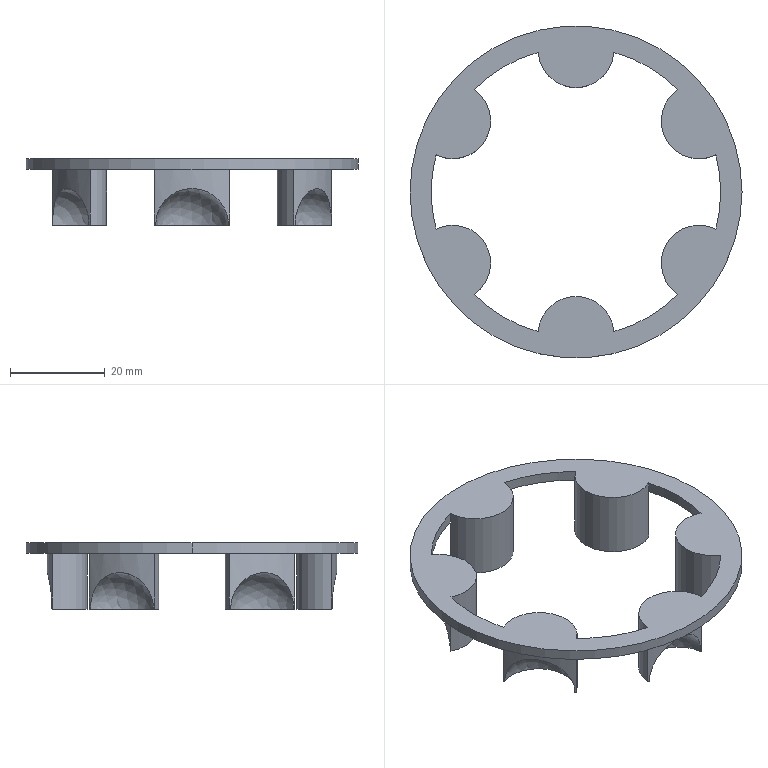Part | NX | features BREP 1 | 1 solid | 37 faces | box 70 x 70 x 14 mm | volume 7900 mm3 | cylinder 23 | plane 8 | sphere 6 | commonest cylinder face diameters 61 x13 16 x8 70 x2
STEP:
#1=CARTESIAN_POINT('',(26.414,15.25,-4.05));
#2=VERTEX_POINT('',#1);
#3=CARTESIAN_POINT('',(21.717,21.415,-11.8));
#4=VERTEX_POINT('',#3);
#5=CARTESIAN_POINT('',(21.717,21.415,-11.8));
#6=CARTESIAN_POINT('',(21.717,21.415,-9.751));
#7=CARTESIAN_POINT('',(22.961,20.244,-5.743));
#8=CARTESIAN_POINT('',(25.389,17.025,-4.05));
#9=CARTESIAN_POINT('',(26.414,15.25,-4.05));
#10=B_SPLINE_CURVE_WITH_KNOTS('',3,(#5,#6,#7,#8,#9),.UNSPECIFIED.,.F.,.F.,(4,1,4),(0.,0.00606,0.01212),.UNSPECIFIED.);
#11=EDGE_CURVE('',#2,#4,#10,.F.);
#12=ORIENTED_EDGE('',*,*,#11,.T.);
#13=CARTESIAN_POINT('',(21.504,21.63,-11.8));
#14=VERTEX_POINT('',#13);
#15=CARTESIAN_POINT('',(0.,0.,-11.8));
#16=DIRECTION('',(0.,0.,-1.));
#17=DIRECTION('',(0.705,0.7092,0.));
#18=AXIS2_PLACEMENT_3D('',#15,#16,#17);
#19=CIRCLE('',#18,30.5);
#20=EDGE_CURVE('',#14,#4,#19,.T.);
#21=ORIENTED_EDGE('',*,*,#20,.F.);
#22=CARTESIAN_POINT('',(21.504,21.63,0.));
#23=VERTEX_POINT('',#22);
#24=CARTESIAN_POINT('',(21.504,21.63,0.));
#25=DIRECTION('',(0.,0.,-1.));
#26=VECTOR('',#25,1000.);
#27=LINE('',#24,#26);
#28=EDGE_CURVE('',#23,#14,#27,.T.);
#29=ORIENTED_EDGE('',*,*,#28,.F.);
#30=CARTESIAN_POINT('',(29.484,7.808,0.));
#31=VERTEX_POINT('',#30);
#32=CARTESIAN_POINT('',(0.,0.,0.));
#33=DIRECTION('',(0.,0.,1.));
#34=DIRECTION('',(0.9667,0.256,0.));
#35=AXIS2_PLACEMENT_3D('',#32,#33,#34);
#36=CIRCLE('',#35,30.5);
#37=EDGE_CURVE('',#31,#23,#36,.T.);
#38=ORIENTED_EDGE('',*,*,#37,.F.);
#39=CARTESIAN_POINT('',(29.484,7.808,-11.8));
#40=VERTEX_POINT('',#39);
#41=CARTESIAN_POINT('',(29.484,7.808,0.));
#42=DIRECTION('',(0.,0.,-1.));
#43=VECTOR('',#42,1000.);
#44=LINE('',#41,#43);
#45=EDGE_CURVE('',#31,#40,#44,.T.);
#46=ORIENTED_EDGE('',*,*,#45,.T.);
#47=CARTESIAN_POINT('',(29.405,8.1,-11.8));
#48=VERTEX_POINT('',#47);
#49=CARTESIAN_POINT('',(0.,0.,-11.8));
#50=DIRECTION('',(0.,0.,-1.));
#51=DIRECTION('',(0.9641,0.2656,0.));
#52=AXIS2_PLACEMENT_3D('',#49,#50,#51);
#53=CIRCLE('',#52,30.5);
#54=EDGE_CURVE('',#48,#40,#53,.T.);
#55=ORIENTED_EDGE('',*,*,#54,.F.);
#56=CARTESIAN_POINT('',(29.405,8.1,-11.8));
#57=CARTESIAN_POINT('',(29.405,8.1,-9.751));
#58=CARTESIAN_POINT('',(29.012,9.763,-5.743));
#59=CARTESIAN_POINT('',(27.439,13.475,-4.05));
#60=CARTESIAN_POINT('',(26.414,15.25,-4.05));
#61=B_SPLINE_CURVE_WITH_KNOTS('',3,(#56,#57,#58,#59,#60),.UNSPECIFIED.,.F.,.F.,(4,1,4),(0.,0.00606,0.01212),.UNSPECIFIED.);
#62=EDGE_CURVE('',#2,#48,#61,.F.);
#63=ORIENTED_EDGE('',*,*,#62,.F.);
#64=EDGE_LOOP('',(#12,#21,#29,#38,#46,#55,#63));
#65=FACE_BOUND('',#64,.T.);
#66=CARTESIAN_POINT('',(0.,0.,-11.8));
#67=DIRECTION('',(0.,0.,1.));
#68=DIRECTION('',(-1.,0.,0.));
#69=AXIS2_PLACEMENT_3D('',#66,#67,#68);
#70=CYLINDRICAL_SURFACE('',#69,30.5);
#71=ADVANCED_FACE('',(#65),#70,.T.);
#72=ORIENTED_EDGE('',*,*,#62,.T.);
#73=CARTESIAN_POINT('',(18.664,15.25,-11.8));
#74=VERTEX_POINT('',#73);
#75=CARTESIAN_POINT('',(26.414,15.25,-11.8));
#76=DIRECTION('',(0.,0.,1.));
#77=DIRECTION('',(-1.,0.,0.));
#78=AXIS2_PLACEMENT_3D('',#75,#76,#77);
#79=CIRCLE('',#78,7.75);
#80=EDGE_CURVE('',#74,#48,#79,.T.);
#81=ORIENTED_EDGE('',*,*,#80,.F.);
#82=CARTESIAN_POINT('',(26.414,15.25,-11.8));
#83=DIRECTION('',(0.,0.,1.));
#84=DIRECTION('',(-0.606,0.7955,0.));
#85=AXIS2_PLACEMENT_3D('',#82,#83,#84);
#86=CIRCLE('',#85,7.75);
#87=EDGE_CURVE('',#4,#74,#86,.T.);
#88=ORIENTED_EDGE('',*,*,#87,.F.);
#89=ORIENTED_EDGE('',*,*,#11,.F.);
#90=EDGE_LOOP('',(#72,#81,#88,#89));
#91=FACE_BOUND('',#90,.T.);
#92=CARTESIAN_POINT('',(26.414,15.25,-11.8));
#93=DIRECTION('',(0.3859,-0.9225,0.));
#94=DIRECTION('',(0.,0.,1.));
#95=AXIS2_PLACEMENT_3D('',#92,#93,#94);
#96=SPHERICAL_SURFACE('',#95,7.75);
#97=ADVANCED_FACE('',(#91),#96,.F.);
#98=ORIENTED_EDGE('',*,*,#87,.T.);
#99=ORIENTED_EDGE('',*,*,#80,.T.);
#100=ORIENTED_EDGE('',*,*,#54,.T.);
#101=CARTESIAN_POINT('',(17.981,15.,-11.8));
#102=VERTEX_POINT('',#101);
#103=CARTESIAN_POINT('',(25.981,15.,-11.8));
#104=DIRECTION('',(0.,0.,-1.));
#105=DIRECTION('',(0.4379,-0.899,0.));
#106=AXIS2_PLACEMENT_3D('',#103,#104,#105);
#107=CIRCLE('',#106,8.);
#108=EDGE_CURVE('',#40,#102,#107,.T.);
#109=ORIENTED_EDGE('',*,*,#108,.T.);
#110=CARTESIAN_POINT('',(25.981,15.,-11.8));
#111=DIRECTION('',(0.,0.,-1.));
#112=DIRECTION('',(-1.,0.,0.));
#113=AXIS2_PLACEMENT_3D('',#110,#111,#112);
#114=CIRCLE('',#113,8.);
#115=EDGE_CURVE('',#102,#14,#114,.T.);
#116=ORIENTED_EDGE('',*,*,#115,.T.);
#117=ORIENTED_EDGE('',*,*,#20,.T.);
#118=EDGE_LOOP('',(#98,#99,#100,#109,#116,#117));
#119=FACE_BOUND('',#118,.T.);
#120=CARTESIAN_POINT('',(12.99,7.5,-11.8));
#121=DIRECTION('',(0.,0.,1.));
#122=DIRECTION('',(-1.,0.,0.));
#123=AXIS2_PLACEMENT_3D('',#120,#121,#122);
#124=PLANE('',#123);
#125=ADVANCED_FACE('',(#119),#124,.F.);
#126=CARTESIAN_POINT('',(21.504,21.63,2.2));
#127=VERTEX_POINT('',#126);
#128=CARTESIAN_POINT('',(17.981,15.,2.2));
#129=VERTEX_POINT('',#128);
#130=CARTESIAN_POINT('',(25.981,15.,2.2));
#131=DIRECTION('',(0.,0.,1.));
#132=DIRECTION('',(-0.5597,0.8287,0.));
#133=AXIS2_PLACEMENT_3D('',#130,#131,#132);
#134=CIRCLE('',#133,8.);
#135=EDGE_CURVE('',#127,#129,#134,.T.);
#136=ORIENTED_EDGE('',*,*,#135,.F.);
#137=CARTESIAN_POINT('',(21.504,21.63,0.));
#138=DIRECTION('',(0.,0.,1.));
#139=VECTOR('',#138,1000.);
#140=LINE('',#137,#139);
#141=EDGE_CURVE('',#23,#127,#140,.T.);
#142=ORIENTED_EDGE('',*,*,#141,.F.);
#143=ORIENTED_EDGE('',*,*,#28,.T.);
#144=ORIENTED_EDGE('',*,*,#115,.F.);
#145=CARTESIAN_POINT('',(17.981,15.,-11.8));
#146=DIRECTION('',(0.,0.,1.));
#147=VECTOR('',#146,1000.);
#148=LINE('',#145,#147);
#149=EDGE_CURVE('',#102,#129,#148,.T.);
#150=ORIENTED_EDGE('',*,*,#149,.T.);
#151=EDGE_LOOP('',(#136,#142,#143,#144,#150));
#152=FACE_BOUND('',#151,.T.);
#153=CARTESIAN_POINT('',(25.981,15.,2.2));
#154=DIRECTION('',(0.,0.,-1.));
#155=DIRECTION('',(1.,0.,0.));
#156=AXIS2_PLACEMENT_3D('',#153,#154,#155);
#157=CYLINDRICAL_SURFACE('',#156,8.);
#158=ADVANCED_FACE('',(#152),#157,.T.);
#159=ORIENTED_EDGE('',*,*,#149,.F.);
#160=ORIENTED_EDGE('',*,*,#108,.F.);
#161=ORIENTED_EDGE('',*,*,#45,.F.);
#162=CARTESIAN_POINT('',(29.484,7.808,2.2));
#163=VERTEX_POINT('',#162);
#164=CARTESIAN_POINT('',(29.484,7.808,0.));
#165=DIRECTION('',(0.,0.,1.));
#166=VECTOR('',#165,1000.);
#167=LINE('',#164,#166);
#168=EDGE_CURVE('',#31,#163,#167,.T.);
#169=ORIENTED_EDGE('',*,*,#168,.T.);
#170=CARTESIAN_POINT('',(25.981,15.,2.2));
#171=DIRECTION('',(0.,0.,1.));
#172=DIRECTION('',(-1.,0.,0.));
#173=AXIS2_PLACEMENT_3D('',#170,#171,#172);
#174=CIRCLE('',#173,8.);
#175=EDGE_CURVE('',#129,#163,#174,.T.);
#176=ORIENTED_EDGE('',*,*,#175,.F.);
#177=EDGE_LOOP('',(#159,#160,#161,#169,#176));
#178=FACE_BOUND('',#177,.T.);
#179=CARTESIAN_POINT('',(25.981,15.,2.2));
#180=DIRECTION('',(0.,0.,-1.));
#181=DIRECTION('',(1.,0.,0.));
#182=AXIS2_PLACEMENT_3D('',#179,#180,#181);
#183=CYLINDRICAL_SURFACE('',#182,8.);
#184=ADVANCED_FACE('',(#178),#183,.T.);
#185=CARTESIAN_POINT('',(35.,0.,2.2));
#186=VERTEX_POINT('',#185);
#187=CARTESIAN_POINT('',(-35.,0.,2.2));
#188=VERTEX_POINT('',#187);
#189=CARTESIAN_POINT('',(0.,0.,2.2));
#190=DIRECTION('',(0.,0.,1.));
#191=DIRECTION('',(1.,0.,0.));
#192=AXIS2_PLACEMENT_3D('',#189,#190,#191);
#193=CIRCLE('',#192,35.);
#194=EDGE_CURVE('',#186,#188,#193,.T.);
#195=ORIENTED_EDGE('',*,*,#194,.T.);
#196=CARTESIAN_POINT('',(0.,0.,2.2));
#197=DIRECTION('',(0.,0.,1.));
#198=DIRECTION('',(-1.,0.,0.));
#199=AXIS2_PLACEMENT_3D('',#196,#197,#198);
#200=CIRCLE('',#199,35.);
#201=EDGE_CURVE('',#188,#186,#200,.T.);
#202=ORIENTED_EDGE('',*,*,#201,.T.);
#203=EDGE_LOOP('',(#195,#202));
#204=FACE_BOUND('',#203,.T.);
#205=CARTESIAN_POINT('',(-29.484,7.808,2.2));
#206=VERTEX_POINT('',#205);
#207=CARTESIAN_POINT('',(-21.504,21.63,2.2));
#208=VERTEX_POINT('',#207);
#209=CARTESIAN_POINT('',(-25.981,15.,2.2));
#210=DIRECTION('',(0.,0.,1.));
#211=DIRECTION('',(-0.4379,-0.899,0.));
#212=AXIS2_PLACEMENT_3D('',#209,#210,#211);
#213=CIRCLE('',#212,8.);
#214=EDGE_CURVE('',#206,#208,#213,.T.);
#215=ORIENTED_EDGE('',*,*,#214,.T.);
#216=CARTESIAN_POINT('',(-7.98,29.438,2.2));
#217=VERTEX_POINT('',#216);
#218=CARTESIAN_POINT('',(0.,0.,2.2));
#219=DIRECTION('',(0.,0.,-1.));
#220=DIRECTION('',(-0.705,0.7092,0.));
#221=AXIS2_PLACEMENT_3D('',#218,#219,#220);
#222=CIRCLE('',#221,30.5);
#223=EDGE_CURVE('',#208,#217,#222,.T.);
#224=ORIENTED_EDGE('',*,*,#223,.T.);
#225=CARTESIAN_POINT('',(7.98,29.438,2.2));
#226=VERTEX_POINT('',#225);
#227=CARTESIAN_POINT('',(0.,30.,2.2));
#228=DIRECTION('',(0.,0.,1.));
#229=DIRECTION('',(-0.9975,-0.07031,0.));
#230=AXIS2_PLACEMENT_3D('',#227,#228,#229);
#231=CIRCLE('',#230,8.);
#232=EDGE_CURVE('',#217,#226,#231,.T.);
#233=ORIENTED_EDGE('',*,*,#232,.T.);
#234=CARTESIAN_POINT('',(0.,0.,2.2));
#235=DIRECTION('',(0.,0.,-1.));
#236=DIRECTION('',(0.2616,0.9652,0.));
#237=AXIS2_PLACEMENT_3D('',#234,#235,#236);
#238=CIRCLE('',#237,30.5);
#239=EDGE_CURVE('',#226,#127,#238,.T.);
#240=ORIENTED_EDGE('',*,*,#239,.T.);
#241=ORIENTED_EDGE('',*,*,#135,.T.);
#242=ORIENTED_EDGE('',*,*,#175,.T.);
#243=CARTESIAN_POINT('',(29.484,-7.808,2.2));
#244=VERTEX_POINT('',#243);
#245=CARTESIAN_POINT('',(0.,0.,2.2));
#246=DIRECTION('',(0.,0.,-1.));
#247=DIRECTION('',(0.9667,0.256,0.));
#248=AXIS2_PLACEMENT_3D('',#245,#246,#247);
#249=CIRCLE('',#248,30.5);
#250=EDGE_CURVE('',#163,#244,#249,.T.);
#251=ORIENTED_EDGE('',*,*,#250,.T.);
#252=CARTESIAN_POINT('',(17.981,-15.,2.2));
#253=VERTEX_POINT('',#252);
#254=CARTESIAN_POINT('',(25.981,-15.,2.2));
#255=DIRECTION('',(0.,0.,1.));
#256=DIRECTION('',(0.4379,0.899,0.));
#257=AXIS2_PLACEMENT_3D('',#254,#255,#256);
#258=CIRCLE('',#257,8.);
#259=EDGE_CURVE('',#244,#253,#258,.T.);
#260=ORIENTED_EDGE('',*,*,#259,.T.);
#261=CARTESIAN_POINT('',(21.504,-21.63,2.2));
#262=VERTEX_POINT('',#261);
#263=CARTESIAN_POINT('',(25.981,-15.,2.2));
#264=DIRECTION('',(0.,0.,1.));
#265=DIRECTION('',(-1.,0.,0.));
#266=AXIS2_PLACEMENT_3D('',#263,#264,#265);
#267=CIRCLE('',#266,8.);
#268=EDGE_CURVE('',#253,#262,#267,.T.);
#269=ORIENTED_EDGE('',*,*,#268,.T.);
#270=CARTESIAN_POINT('',(7.98,-29.438,2.2));
#271=VERTEX_POINT('',#270);
#272=CARTESIAN_POINT('',(0.,0.,2.2));
#273=DIRECTION('',(0.,0.,-1.));
#274=DIRECTION('',(0.705,-0.7092,0.));
#275=AXIS2_PLACEMENT_3D('',#272,#273,#274);
#276=CIRCLE('',#275,30.5);
#277=EDGE_CURVE('',#262,#271,#276,.T.);
#278=ORIENTED_EDGE('',*,*,#277,.T.);
#279=CARTESIAN_POINT('',(-7.98,-29.438,2.2));
#280=VERTEX_POINT('',#279);
#281=CARTESIAN_POINT('',(0.,-30.,2.2));
#282=DIRECTION('',(0.,0.,1.));
#283=DIRECTION('',(0.9975,0.07031,0.));
#284=AXIS2_PLACEMENT_3D('',#281,#282,#283);
#285=CIRCLE('',#284,8.);
#286=EDGE_CURVE('',#271,#280,#285,.T.);
#287=ORIENTED_EDGE('',*,*,#286,.T.);
#288=CARTESIAN_POINT('',(-21.504,-21.63,2.2));
#289=VERTEX_POINT('',#288);
#290=CARTESIAN_POINT('',(0.,0.,2.2));
#291=DIRECTION('',(0.,0.,-1.));
#292=DIRECTION('',(-0.2616,-0.9652,0.));
#293=AXIS2_PLACEMENT_3D('',#290,#291,#292);
#294=CIRCLE('',#293,30.5);
#295=EDGE_CURVE('',#280,#289,#294,.T.);
#296=ORIENTED_EDGE('',*,*,#295,.T.);
#297=CARTESIAN_POINT('',(-29.484,-7.808,2.2));
#298=VERTEX_POINT('',#297);
#299=CARTESIAN_POINT('',(-25.981,-15.,2.2));
#300=DIRECTION('',(0.,0.,1.));
#301=DIRECTION('',(0.5597,-0.8287,0.));
#302=AXIS2_PLACEMENT_3D('',#299,#300,#301);
#303=CIRCLE('',#302,8.);
#304=EDGE_CURVE('',#289,#298,#303,.T.);
#305=ORIENTED_EDGE('',*,*,#304,.T.);
#306=CARTESIAN_POINT('',(-30.5,0.,2.2));
#307=VERTEX_POINT('',#306);
#308=CARTESIAN_POINT('',(0.,0.,2.2));
#309=DIRECTION('',(0.,0.,-1.));
#310=DIRECTION('',(-0.9667,-0.256,0.));
#311=AXIS2_PLACEMENT_3D('',#308,#309,#310);
#312=CIRCLE('',#311,30.5);
#313=EDGE_CURVE('',#298,#307,#312,.T.);
#314=ORIENTED_EDGE('',*,*,#313,.T.);
#315=CARTESIAN_POINT('',(0.,0.,2.2));
#316=DIRECTION('',(0.,0.,-1.));
#317=DIRECTION('',(-1.,0.,0.));
#318=AXIS2_PLACEMENT_3D('',#315,#316,#317);
#319=CIRCLE('',#318,30.5);
#320=EDGE_CURVE('',#307,#206,#319,.T.);
#321=ORIENTED_EDGE('',*,*,#320,.T.);
#322=EDGE_LOOP('',(#215,#224,#233,#240,#241,#242,#251,#260,#269,#278,#287,#296,#305,#314,#321));
#323=FACE_BOUND('',#322,.T.);
#324=CARTESIAN_POINT('',(0.,0.,2.2));
#325=DIRECTION('',(0.,0.,1.));
#326=DIRECTION('',(-1.,0.,0.));
#327=AXIS2_PLACEMENT_3D('',#324,#325,#326);
#328=PLANE('',#327);
#329=ADVANCED_FACE('',(#204,#323),#328,.T.);
#330=ORIENTED_EDGE('',*,*,#201,.F.);
#331=CARTESIAN_POINT('',(-35.,0.,0.));
#332=VERTEX_POINT('',#331);
#333=CARTESIAN_POINT('',(-35.,0.,0.));
#334=DIRECTION('',(0.,0.,1.));
#335=VECTOR('',#334,1000.);
#336=LINE('',#333,#335);
#337=EDGE_CURVE('',#188,#332,#336,.F.);
#338=ORIENTED_EDGE('',*,*,#337,.T.);
#339=CARTESIAN_POINT('',(35.,0.,0.));
#340=VERTEX_POINT('',#339);
#341=CARTESIAN_POINT('',(0.,0.,0.));
#342=DIRECTION('',(0.,0.,-1.));
#343=DIRECTION('',(1.,0.,0.));
#344=AXIS2_PLACEMENT_3D('',#341,#342,#343);
#345=CIRCLE('',#344,35.);
#346=EDGE_CURVE('',#340,#332,#345,.T.);
#347=ORIENTED_EDGE('',*,*,#346,.F.);
#348=CARTESIAN_POINT('',(35.,0.,0.));
#349=DIRECTION('',(0.,0.,1.));
#350=VECTOR('',#349,1000.);
#351=LINE('',#348,#350);
#352=EDGE_CURVE('',#186,#340,#351,.F.);
#353=ORIENTED_EDGE('',*,*,#352,.F.);
#354=EDGE_LOOP('',(#330,#338,#347,#353));
#355=FACE_BOUND('',#354,.T.);
#356=CARTESIAN_POINT('',(0.,0.,2.2));
#357=DIRECTION('',(0.,0.,-1.));
#358=DIRECTION('',(1.,0.,0.));
#359=AXIS2_PLACEMENT_3D('',#356,#357,#358);
#360=CYLINDRICAL_SURFACE('',#359,35.);
#361=ADVANCED_FACE('',(#355),#360,.T.);
#362=ORIENTED_EDGE('',*,*,#352,.T.);
#363=CARTESIAN_POINT('',(0.,0.,0.));
#364=DIRECTION('',(0.,0.,-1.));
#365=DIRECTION('',(-1.,0.,0.));
#366=AXIS2_PLACEMENT_3D('',#363,#364,#365);
#367=CIRCLE('',#366,35.);
#368=EDGE_CURVE('',#332,#340,#367,.T.);
#369=ORIENTED_EDGE('',*,*,#368,.F.);
#370=ORIENTED_EDGE('',*,*,#337,.F.);
#371=ORIENTED_EDGE('',*,*,#194,.F.);
#372=EDGE_LOOP('',(#362,#369,#370,#371));
#373=FACE_BOUND('',#372,.T.);
#374=CARTESIAN_POINT('',(0.,0.,2.2));
#375=DIRECTION('',(0.,0.,-1.));
#376=DIRECTION('',(1.,0.,0.));
#377=AXIS2_PLACEMENT_3D('',#374,#375,#376);
#378=CYLINDRICAL_SURFACE('',#377,35.);
#379=ADVANCED_FACE('',(#373),#378,.T.);
#380=ORIENTED_EDGE('',*,*,#368,.T.);
#381=ORIENTED_EDGE('',*,*,#346,.T.);
#382=EDGE_LOOP('',(#380,#381));
#383=FACE_BOUND('',#382,.T.);
#384=CARTESIAN_POINT('',(-21.504,21.63,0.));
#385=VERTEX_POINT('',#384);
#386=CARTESIAN_POINT('',(-29.484,7.808,0.));
#387=VERTEX_POINT('',#386);
#388=CARTESIAN_POINT('',(0.,0.,0.));
#389=DIRECTION('',(0.,0.,1.));
#390=DIRECTION('',(-0.705,0.7092,0.));
#391=AXIS2_PLACEMENT_3D('',#388,#389,#390);
#392=CIRCLE('',#391,30.5);
#393=EDGE_CURVE('',#385,#387,#392,.T.);
#394=ORIENTED_EDGE('',*,*,#393,.T.);
#395=CARTESIAN_POINT('',(-30.5,0.,0.));
#396=VERTEX_POINT('',#395);
#397=CARTESIAN_POINT('',(0.,0.,0.));
#398=DIRECTION('',(0.,0.,1.));
#399=DIRECTION('',(-0.9667,0.256,0.));
#400=AXIS2_PLACEMENT_3D('',#397,#398,#399);
#401=CIRCLE('',#400,30.5);
#402=EDGE_CURVE('',#387,#396,#401,.T.);
#403=ORIENTED_EDGE('',*,*,#402,.T.);
#404=CARTESIAN_POINT('',(-29.484,-7.808,0.));
#405=VERTEX_POINT('',#404);
#406=CARTESIAN_POINT('',(0.,0.,0.));
#407=DIRECTION('',(0.,0.,1.));
#408=DIRECTION('',(-1.,0.,0.));
#409=AXIS2_PLACEMENT_3D('',#406,#407,#408);
#410=CIRCLE('',#409,30.5);
#411=EDGE_CURVE('',#396,#405,#410,.T.);
#412=ORIENTED_EDGE('',*,*,#411,.T.);
#413=CARTESIAN_POINT('',(-21.504,-21.63,0.));
#414=VERTEX_POINT('',#413);
#415=CARTESIAN_POINT('',(0.,0.,0.));
#416=DIRECTION('',(0.,0.,1.));
#417=DIRECTION('',(-0.9667,-0.256,0.));
#418=AXIS2_PLACEMENT_3D('',#415,#416,#417);
#419=CIRCLE('',#418,30.5);
#420=EDGE_CURVE('',#405,#414,#419,.T.);
#421=ORIENTED_EDGE('',*,*,#420,.T.);
#422=CARTESIAN_POINT('',(-7.98,-29.438,0.));
#423=VERTEX_POINT('',#422);
#424=CARTESIAN_POINT('',(0.,0.,0.));
#425=DIRECTION('',(0.,0.,1.));
#426=DIRECTION('',(-0.705,-0.7092,0.));
#427=AXIS2_PLACEMENT_3D('',#424,#425,#426);
#428=CIRCLE('',#427,30.5);
#429=EDGE_CURVE('',#414,#423,#428,.T.);
#430=ORIENTED_EDGE('',*,*,#429,.T.);
#431=CARTESIAN_POINT('',(7.98,-29.438,0.));
#432=VERTEX_POINT('',#431);
#433=CARTESIAN_POINT('',(0.,0.,0.));
#434=DIRECTION('',(0.,0.,1.));
#435=DIRECTION('',(-0.2616,-0.9652,0.));
#436=AXIS2_PLACEMENT_3D('',#433,#434,#435);
#437=CIRCLE('',#436,30.5);
#438=EDGE_CURVE('',#423,#432,#437,.T.);
#439=ORIENTED_EDGE('',*,*,#438,.T.);
#440=CARTESIAN_POINT('',(21.504,-21.63,0.));
#441=VERTEX_POINT('',#440);
#442=CARTESIAN_POINT('',(0.,0.,0.));
#443=DIRECTION('',(0.,0.,1.));
#444=DIRECTION('',(0.2616,-0.9652,0.));
#445=AXIS2_PLACEMENT_3D('',#442,#443,#444);
#446=CIRCLE('',#445,30.5);
#447=EDGE_CURVE('',#432,#441,#446,.T.);
#448=ORIENTED_EDGE('',*,*,#447,.T.);
#449=CARTESIAN_POINT('',(29.484,-7.808,0.));
#450=VERTEX_POINT('',#449);
#451=CARTESIAN_POINT('',(0.,0.,0.));
#452=DIRECTION('',(0.,0.,1.));
#453=DIRECTION('',(0.705,-0.7092,0.));
#454=AXIS2_PLACEMENT_3D('',#451,#452,#453);
#455=CIRCLE('',#454,30.5);
#456=EDGE_CURVE('',#441,#450,#455,.T.);
#457=ORIENTED_EDGE('',*,*,#456,.T.);
#458=CARTESIAN_POINT('',(0.,0.,0.));
#459=DIRECTION('',(0.,0.,1.));
#460=DIRECTION('',(0.9667,-0.256,0.));
#461=AXIS2_PLACEMENT_3D('',#458,#459,#460);
#462=CIRCLE('',#461,30.5);
#463=EDGE_CURVE('',#450,#31,#462,.T.);
#464=ORIENTED_EDGE('',*,*,#463,.T.);
#465=ORIENTED_EDGE('',*,*,#37,.T.);
#466=CARTESIAN_POINT('',(7.98,29.438,0.));
#467=VERTEX_POINT('',#466);
#468=CARTESIAN_POINT('',(0.,0.,0.));
#469=DIRECTION('',(0.,0.,1.));
#470=DIRECTION('',(0.705,0.7092,0.));
#471=AXIS2_PLACEMENT_3D('',#468,#469,#470);
#472=CIRCLE('',#471,30.5);
#473=EDGE_CURVE('',#23,#467,#472,.T.);
#474=ORIENTED_EDGE('',*,*,#473,.T.);
#475=CARTESIAN_POINT('',(-7.98,29.438,0.));
#476=VERTEX_POINT('',#475);
#477=CARTESIAN_POINT('',(0.,0.,0.));
#478=DIRECTION('',(0.,0.,1.));
#479=DIRECTION('',(0.2616,0.9652,0.));
#480=AXIS2_PLACEMENT_3D('',#477,#478,#479);
#481=CIRCLE('',#480,30.5);
#482=EDGE_CURVE('',#467,#476,#481,.T.);
#483=ORIENTED_EDGE('',*,*,#482,.T.);
#484=CARTESIAN_POINT('',(0.,0.,0.));
#485=DIRECTION('',(0.,0.,1.));
#486=DIRECTION('',(-0.2616,0.9652,0.));
#487=AXIS2_PLACEMENT_3D('',#484,#485,#486);
#488=CIRCLE('',#487,30.5);
#489=EDGE_CURVE('',#476,#385,#488,.T.);
#490=ORIENTED_EDGE('',*,*,#489,.T.);
#491=EDGE_LOOP('',(#394,#403,#412,#421,#430,#439,#448,#457,#464,#465,#474,#483,#490));
#492=FACE_BOUND('',#491,.T.);
#493=CARTESIAN_POINT('',(0.,0.,0.));
#494=DIRECTION('',(0.,0.,1.));
#495=DIRECTION('',(-1.,0.,0.));
#496=AXIS2_PLACEMENT_3D('',#493,#494,#495);
#497=PLANE('',#496);
#498=ADVANCED_FACE('',(#383,#492),#497,.F.);
#499=CARTESIAN_POINT('',(-7.98,29.438,0.));
#500=DIRECTION('',(0.,0.,1.));
#501=VECTOR('',#500,1000.);
#502=LINE('',#499,#501);
#503=EDGE_CURVE('',#476,#217,#502,.T.);
#504=ORIENTED_EDGE('',*,*,#503,.T.);
#505=ORIENTED_EDGE('',*,*,#223,.F.);
#506=CARTESIAN_POINT('',(-21.504,21.63,0.));
#507=DIRECTION('',(0.,0.,1.));
#508=VECTOR('',#507,1000.);
#509=LINE('',#506,#508);
#510=EDGE_CURVE('',#385,#208,#509,.T.);
#511=ORIENTED_EDGE('',*,*,#510,.F.);
#512=ORIENTED_EDGE('',*,*,#489,.F.);
#513=EDGE_LOOP('',(#504,#505,#511,#512));
#514=FACE_BOUND('',#513,.T.);
#515=CARTESIAN_POINT('',(0.,0.,2.2));
#516=DIRECTION('',(0.,0.,-1.));
#517=DIRECTION('',(1.,0.,0.));
#518=AXIS2_PLACEMENT_3D('',#515,#516,#517);
#519=CYLINDRICAL_SURFACE('',#518,30.5);
#520=ADVANCED_FACE('',(#514),#519,.F.);
#521=CARTESIAN_POINT('',(-29.484,7.808,-11.8));
#522=VERTEX_POINT('',#521);
#523=CARTESIAN_POINT('',(-29.484,7.808,0.));
#524=DIRECTION('',(0.,0.,-1.));
#525=VECTOR('',#524,1000.);
#526=LINE('',#523,#525);
#527=EDGE_CURVE('',#387,#522,#526,.T.);
#528=ORIENTED_EDGE('',*,*,#527,.T.);
#529=CARTESIAN_POINT('',(-21.504,21.63,-11.8));
#530=VERTEX_POINT('',#529);
#531=CARTESIAN_POINT('',(-25.981,15.,-11.8));
#532=DIRECTION('',(0.,0.,-1.));
#533=DIRECTION('',(0.5597,0.8287,0.));
#534=AXIS2_PLACEMENT_3D('',#531,#532,#533);
#535=CIRCLE('',#534,8.);
#536=EDGE_CURVE('',#530,#522,#535,.T.);
#537=ORIENTED_EDGE('',*,*,#536,.F.);
#538=CARTESIAN_POINT('',(-21.504,21.63,0.));
#539=DIRECTION('',(0.,0.,-1.));
#540=VECTOR('',#539,1000.);
#541=LINE('',#538,#540);
#542=EDGE_CURVE('',#385,#530,#541,.T.);
#543=ORIENTED_EDGE('',*,*,#542,.F.);
#544=ORIENTED_EDGE('',*,*,#510,.T.);
#545=ORIENTED_EDGE('',*,*,#214,.F.);
#546=CARTESIAN_POINT('',(-29.484,7.808,0.));
#547=DIRECTION('',(0.,0.,1.));
#548=VECTOR('',#547,1000.);
#549=LINE('',#546,#548);
#550=EDGE_CURVE('',#387,#206,#549,.T.);
#551=ORIENTED_EDGE('',*,*,#550,.F.);
#552=EDGE_LOOP('',(#528,#537,#543,#544,#545,#551));
#553=FACE_BOUND('',#552,.T.);
#554=CARTESIAN_POINT('',(-25.981,15.,2.2));
#555=DIRECTION('',(0.,0.,-1.));
#556=DIRECTION('',(1.,0.,0.));
#557=AXIS2_PLACEMENT_3D('',#554,#555,#556);
#558=CYLINDRICAL_SURFACE('',#557,8.);
#559=ADVANCED_FACE('',(#553),#558,.T.);
#560=CARTESIAN_POINT('',(-30.5,0.,0.));
#561=DIRECTION('',(0.,0.,1.));
#562=VECTOR('',#561,1000.);
#563=LINE('',#560,#562);
#564=EDGE_CURVE('',#396,#307,#563,.T.);
#565=ORIENTED_EDGE('',*,*,#564,.F.);
#566=ORIENTED_EDGE('',*,*,#402,.F.);
#567=ORIENTED_EDGE('',*,*,#550,.T.);
#568=ORIENTED_EDGE('',*,*,#320,.F.);
#569=EDGE_LOOP('',(#565,#566,#567,#568));
#570=FACE_BOUND('',#569,.T.);
#571=CARTESIAN_POINT('',(0.,0.,2.2));
#572=DIRECTION('',(0.,0.,-1.));
#573=DIRECTION('',(1.,0.,0.));
#574=AXIS2_PLACEMENT_3D('',#571,#572,#573);
#575=CYLINDRICAL_SURFACE('',#574,30.5);
#576=ADVANCED_FACE('',(#570),#575,.F.);
#577=ORIENTED_EDGE('',*,*,#313,.F.);
#578=CARTESIAN_POINT('',(-29.484,-7.808,0.));
#579=DIRECTION('',(0.,0.,1.));
#580=VECTOR('',#579,1000.);
#581=LINE('',#578,#580);
#582=EDGE_CURVE('',#405,#298,#581,.T.);
#583=ORIENTED_EDGE('',*,*,#582,.F.);
#584=ORIENTED_EDGE('',*,*,#411,.F.);
#585=ORIENTED_EDGE('',*,*,#564,.T.);
#586=EDGE_LOOP('',(#577,#583,#584,#585));
#587=FACE_BOUND('',#586,.T.);
#588=CARTESIAN_POINT('',(0.,0.,2.2));
#589=DIRECTION('',(0.,0.,-1.));
#590=DIRECTION('',(1.,0.,0.));
#591=AXIS2_PLACEMENT_3D('',#588,#589,#590);
#592=CYLINDRICAL_SURFACE('',#591,30.5);
#593=ADVANCED_FACE('',(#587),#592,.F.);
#594=CARTESIAN_POINT('',(-21.504,-21.63,-11.8));
#595=VERTEX_POINT('',#594);
#596=CARTESIAN_POINT('',(-21.504,-21.63,0.));
#597=DIRECTION('',(0.,0.,-1.));
#598=VECTOR('',#597,1000.);
#599=LINE('',#596,#598);
#600=EDGE_CURVE('',#595,#414,#599,.F.);
#601=ORIENTED_EDGE('',*,*,#600,.F.);
#602=CARTESIAN_POINT('',(-29.484,-7.808,-11.8));
#603=VERTEX_POINT('',#602);
#604=CARTESIAN_POINT('',(-25.981,-15.,-11.8));
#605=DIRECTION('',(0.,0.,-1.));
#606=DIRECTION('',(-0.4379,0.899,0.));
#607=AXIS2_PLACEMENT_3D('',#604,#605,#606);
#608=CIRCLE('',#607,8.);
#609=EDGE_CURVE('',#603,#595,#608,.T.);
#610=ORIENTED_EDGE('',*,*,#609,.F.);
#611=CARTESIAN_POINT('',(-29.484,-7.808,0.));
#612=DIRECTION('',(0.,0.,-1.));
#613=VECTOR('',#612,1000.);
#614=LINE('',#611,#613);
#615=EDGE_CURVE('',#603,#405,#614,.F.);
#616=ORIENTED_EDGE('',*,*,#615,.T.);
#617=ORIENTED_EDGE('',*,*,#582,.T.);
#618=ORIENTED_EDGE('',*,*,#304,.F.);
#619=CARTESIAN_POINT('',(-21.504,-21.63,0.));
#620=DIRECTION('',(0.,0.,1.));
#621=VECTOR('',#620,1000.);
#622=LINE('',#619,#621);
#623=EDGE_CURVE('',#414,#289,#622,.T.);
#624=ORIENTED_EDGE('',*,*,#623,.F.);
#625=EDGE_LOOP('',(#601,#610,#616,#617,#618,#624));
#626=FACE_BOUND('',#625,.T.);
#627=CARTESIAN_POINT('',(-25.981,-15.,2.2));
#628=DIRECTION('',(0.,0.,-1.));
#629=DIRECTION('',(1.,0.,0.));
#630=AXIS2_PLACEMENT_3D('',#627,#628,#629);
#631=CYLINDRICAL_SURFACE('',#630,8.);
#632=ADVANCED_FACE('',(#626),#631,.T.);
#633=ORIENTED_EDGE('',*,*,#623,.T.);
#634=ORIENTED_EDGE('',*,*,#295,.F.);
#635=CARTESIAN_POINT('',(-7.98,-29.438,0.));
#636=DIRECTION('',(0.,0.,1.));
#637=VECTOR('',#636,1000.);
#638=LINE('',#635,#637);
#639=EDGE_CURVE('',#423,#280,#638,.T.);
#640=ORIENTED_EDGE('',*,*,#639,.F.);
#641=ORIENTED_EDGE('',*,*,#429,.F.);
#642=EDGE_LOOP('',(#633,#634,#640,#641));
#643=FACE_BOUND('',#642,.T.);
#644=CARTESIAN_POINT('',(0.,0.,2.2));
#645=DIRECTION('',(0.,0.,-1.));
#646=DIRECTION('',(1.,0.,0.));
#647=AXIS2_PLACEMENT_3D('',#644,#645,#646);
#648=CYLINDRICAL_SURFACE('',#647,30.5);
#649=ADVANCED_FACE('',(#643),#648,.F.);
#650=CARTESIAN_POINT('',(7.98,-29.438,-11.8));
#651=VERTEX_POINT('',#650);
#652=CARTESIAN_POINT('',(7.98,-29.438,0.));
#653=DIRECTION('',(0.,0.,-1.));
#654=VECTOR('',#653,1000.);
#655=LINE('',#652,#654);
#656=EDGE_CURVE('',#651,#432,#655,.F.);
#657=ORIENTED_EDGE('',*,*,#656,.F.);
#658=CARTESIAN_POINT('',(-7.98,-29.438,-11.8));
#659=VERTEX_POINT('',#658);
#660=CARTESIAN_POINT('',(0.,-30.,-11.8));
#661=DIRECTION('',(0.,0.,-1.));
#662=DIRECTION('',(-0.9975,0.07031,0.));
#663=AXIS2_PLACEMENT_3D('',#660,#661,#662);
#664=CIRCLE('',#663,8.);
#665=EDGE_CURVE('',#659,#651,#664,.T.);
#666=ORIENTED_EDGE('',*,*,#665,.F.);
#667=CARTESIAN_POINT('',(-7.98,-29.438,0.));
#668=DIRECTION('',(0.,0.,-1.));
#669=VECTOR('',#668,1000.);
#670=LINE('',#667,#669);
#671=EDGE_CURVE('',#659,#423,#670,.F.);
#672=ORIENTED_EDGE('',*,*,#671,.T.);
#673=ORIENTED_EDGE('',*,*,#639,.T.);
#674=ORIENTED_EDGE('',*,*,#286,.F.);
#675=CARTESIAN_POINT('',(7.98,-29.438,0.));
#676=DIRECTION('',(0.,0.,1.));
#677=VECTOR('',#676,1000.);
#678=LINE('',#675,#677);
#679=EDGE_CURVE('',#432,#271,#678,.T.);
#680=ORIENTED_EDGE('',*,*,#679,.F.);
#681=EDGE_LOOP('',(#657,#666,#672,#673,#674,#680));
#682=FACE_BOUND('',#681,.T.);
#683=CARTESIAN_POINT('',(0.,-30.,2.2));
#684=DIRECTION('',(0.,0.,-1.));
#685=DIRECTION('',(1.,0.,0.));
#686=AXIS2_PLACEMENT_3D('',#683,#684,#685);
#687=CYLINDRICAL_SURFACE('',#686,8.);
#688=ADVANCED_FACE('',(#682),#687,.T.);
#689=ORIENTED_EDGE('',*,*,#679,.T.);
#690=ORIENTED_EDGE('',*,*,#277,.F.);
#691=CARTESIAN_POINT('',(21.504,-21.63,0.));
#692=DIRECTION('',(0.,0.,1.));
#693=VECTOR('',#692,1000.);
#694=LINE('',#691,#693);
#695=EDGE_CURVE('',#441,#262,#694,.T.);
#696=ORIENTED_EDGE('',*,*,#695,.F.);
#697=ORIENTED_EDGE('',*,*,#447,.F.);
#698=EDGE_LOOP('',(#689,#690,#696,#697));
#699=FACE_BOUND('',#698,.T.);
#700=CARTESIAN_POINT('',(0.,0.,2.2));
#701=DIRECTION('',(0.,0.,-1.));
#702=DIRECTION('',(1.,0.,0.));
#703=AXIS2_PLACEMENT_3D('',#700,#701,#702);
#704=CYLINDRICAL_SURFACE('',#703,30.5);
#705=ADVANCED_FACE('',(#699),#704,.F.);
#706=CARTESIAN_POINT('',(17.981,-15.,-11.8));
#707=VERTEX_POINT('',#706);
#708=CARTESIAN_POINT('',(17.981,-15.,-11.8));
#709=DIRECTION('',(0.,0.,1.));
#710=VECTOR('',#709,1000.);
#711=LINE('',#708,#710);
#712=EDGE_CURVE('',#707,#253,#711,.T.);
#713=ORIENTED_EDGE('',*,*,#712,.F.);
#714=CARTESIAN_POINT('',(21.504,-21.63,-11.8));
#715=VERTEX_POINT('',#714);
#716=CARTESIAN_POINT('',(25.981,-15.,-11.8));
#717=DIRECTION('',(0.,0.,-1.));
#718=DIRECTION('',(-0.5597,-0.8287,0.));
#719=AXIS2_PLACEMENT_3D('',#716,#717,#718);
#720=CIRCLE('',#719,8.);
#721=EDGE_CURVE('',#715,#707,#720,.T.);
#722=ORIENTED_EDGE('',*,*,#721,.F.);
#723=CARTESIAN_POINT('',(21.504,-21.63,0.));
#724=DIRECTION('',(0.,0.,-1.));
#725=VECTOR('',#724,1000.);
#726=LINE('',#723,#725);
#727=EDGE_CURVE('',#441,#715,#726,.T.);
#728=ORIENTED_EDGE('',*,*,#727,.F.);
#729=ORIENTED_EDGE('',*,*,#695,.T.);
#730=ORIENTED_EDGE('',*,*,#268,.F.);
#731=EDGE_LOOP('',(#713,#722,#728,#729,#730));
#732=FACE_BOUND('',#731,.T.);
#733=CARTESIAN_POINT('',(25.981,-15.,2.2));
#734=DIRECTION('',(0.,0.,-1.));
#735=DIRECTION('',(1.,0.,0.));
#736=AXIS2_PLACEMENT_3D('',#733,#734,#735);
#737=CYLINDRICAL_SURFACE('',#736,8.);
#738=ADVANCED_FACE('',(#732),#737,.T.);
#739=CARTESIAN_POINT('',(29.405,-8.1,-11.8));
#740=VERTEX_POINT('',#739);
#741=CARTESIAN_POINT('',(26.414,-15.25,-4.05));
#742=VERTEX_POINT('',#741);
#743=CARTESIAN_POINT('',(29.405,-8.1,-11.8));
#744=CARTESIAN_POINT('',(29.405,-8.1,-9.751));
#745=CARTESIAN_POINT('',(29.012,-9.763,-5.743));
#746=CARTESIAN_POINT('',(27.439,-13.475,-4.05));
#747=CARTESIAN_POINT('',(26.414,-15.25,-4.05));
#748=B_SPLINE_CURVE_WITH_KNOTS('',3,(#743,#744,#745,#746,#747),.UNSPECIFIED.,.F.,.F.,(4,1,4),(0.,0.00606,0.01212),.UNSPECIFIED.);
#749=EDGE_CURVE('',#740,#742,#748,.T.);
#750=ORIENTED_EDGE('',*,*,#749,.F.);
#751=CARTESIAN_POINT('',(29.484,-7.808,-11.8));
#752=VERTEX_POINT('',#751);
#753=CARTESIAN_POINT('',(0.,0.,-11.8));
#754=DIRECTION('',(0.,0.,-1.));
#755=DIRECTION('',(0.9667,-0.256,0.));
#756=AXIS2_PLACEMENT_3D('',#753,#754,#755);
#757=CIRCLE('',#756,30.5);
#758=EDGE_CURVE('',#752,#740,#757,.T.);
#759=ORIENTED_EDGE('',*,*,#758,.F.);
#760=CARTESIAN_POINT('',(29.484,-7.808,0.));
#761=DIRECTION('',(0.,0.,-1.));
#762=VECTOR('',#761,1000.);
#763=LINE('',#760,#762);
#764=EDGE_CURVE('',#450,#752,#763,.T.);
#765=ORIENTED_EDGE('',*,*,#764,.F.);
#766=ORIENTED_EDGE('',*,*,#456,.F.);
#767=ORIENTED_EDGE('',*,*,#727,.T.);
#768=CARTESIAN_POINT('',(21.717,-21.415,-11.8));
#769=VERTEX_POINT('',#768);
#770=CARTESIAN_POINT('',(0.,0.,-11.8));
#771=DIRECTION('',(0.,0.,-1.));
#772=DIRECTION('',(0.712,-0.7021,0.));
#773=AXIS2_PLACEMENT_3D('',#770,#771,#772);
#774=CIRCLE('',#773,30.5);
#775=EDGE_CURVE('',#769,#715,#774,.T.);
#776=ORIENTED_EDGE('',*,*,#775,.F.);
#777=CARTESIAN_POINT('',(21.717,-21.415,-11.8));
#778=CARTESIAN_POINT('',(21.717,-21.415,-9.751));
#779=CARTESIAN_POINT('',(22.961,-20.244,-5.743));
#780=CARTESIAN_POINT('',(25.389,-17.025,-4.05));
#781=CARTESIAN_POINT('',(26.414,-15.25,-4.05));
#782=B_SPLINE_CURVE_WITH_KNOTS('',3,(#777,#778,#779,#780,#781),.UNSPECIFIED.,.F.,.F.,(4,1,4),(0.,0.00606,0.01212),.UNSPECIFIED.);
#783=EDGE_CURVE('',#769,#742,#782,.T.);
#784=ORIENTED_EDGE('',*,*,#783,.T.);
#785=EDGE_LOOP('',(#750,#759,#765,#766,#767,#776,#784));
#786=FACE_BOUND('',#785,.T.);
#787=CARTESIAN_POINT('',(0.,0.,-11.8));
#788=DIRECTION('',(0.,0.,1.));
#789=DIRECTION('',(-1.,0.,0.));
#790=AXIS2_PLACEMENT_3D('',#787,#788,#789);
#791=CYLINDRICAL_SURFACE('',#790,30.5);
#792=ADVANCED_FACE('',(#786),#791,.T.);
#793=ORIENTED_EDGE('',*,*,#783,.F.);
#794=CARTESIAN_POINT('',(18.664,-15.25,-11.8));
#795=VERTEX_POINT('',#794);
#796=CARTESIAN_POINT('',(26.414,-15.25,-11.8));
#797=DIRECTION('',(0.,0.,1.));
#798=DIRECTION('',(-1.,0.,0.));
#799=AXIS2_PLACEMENT_3D('',#796,#797,#798);
#800=CIRCLE('',#799,7.75);
#801=EDGE_CURVE('',#795,#769,#800,.T.);
#802=ORIENTED_EDGE('',*,*,#801,.F.);
#803=CARTESIAN_POINT('',(26.414,-15.25,-11.8));
#804=DIRECTION('',(0.,0.,1.));
#805=DIRECTION('',(0.3859,0.9225,0.));
#806=AXIS2_PLACEMENT_3D('',#803,#804,#805);
#807=CIRCLE('',#806,7.75);
#808=EDGE_CURVE('',#740,#795,#807,.T.);
#809=ORIENTED_EDGE('',*,*,#808,.F.);
#810=ORIENTED_EDGE('',*,*,#749,.T.);
#811=EDGE_LOOP('',(#793,#802,#809,#810));
#812=FACE_BOUND('',#811,.T.);
#813=CARTESIAN_POINT('',(26.414,-15.25,-11.8));
#814=DIRECTION('',(-0.606,-0.7955,0.));
#815=DIRECTION('',(0.,0.,1.));
#816=AXIS2_PLACEMENT_3D('',#813,#814,#815);
#817=SPHERICAL_SURFACE('',#816,7.75);
#818=ADVANCED_FACE('',(#812),#817,.F.);
#819=ORIENTED_EDGE('',*,*,#808,.T.);
#820=ORIENTED_EDGE('',*,*,#801,.T.);
#821=ORIENTED_EDGE('',*,*,#775,.T.);
#822=ORIENTED_EDGE('',*,*,#721,.T.);
#823=CARTESIAN_POINT('',(25.981,-15.,-11.8));
#824=DIRECTION('',(0.,0.,-1.));
#825=DIRECTION('',(-1.,0.,0.));
#826=AXIS2_PLACEMENT_3D('',#823,#824,#825);
#827=CIRCLE('',#826,8.);
#828=EDGE_CURVE('',#707,#752,#827,.T.);
#829=ORIENTED_EDGE('',*,*,#828,.T.);
#830=ORIENTED_EDGE('',*,*,#758,.T.);
#831=EDGE_LOOP('',(#819,#820,#821,#822,#829,#830));
#832=FACE_BOUND('',#831,.T.);
#833=CARTESIAN_POINT('',(12.99,-7.5,-11.8));
#834=DIRECTION('',(0.,0.,1.));
#835=DIRECTION('',(-1.,0.,0.));
#836=AXIS2_PLACEMENT_3D('',#833,#834,#835);
#837=PLANE('',#836);
#838=ADVANCED_FACE('',(#832),#837,.F.);
#839=ORIENTED_EDGE('',*,*,#259,.F.);
#840=CARTESIAN_POINT('',(29.484,-7.808,0.));
#841=DIRECTION('',(0.,0.,1.));
#842=VECTOR('',#841,1000.);
#843=LINE('',#840,#842);
#844=EDGE_CURVE('',#450,#244,#843,.T.);
#845=ORIENTED_EDGE('',*,*,#844,.F.);
#846=ORIENTED_EDGE('',*,*,#764,.T.);
#847=ORIENTED_EDGE('',*,*,#828,.F.);
#848=ORIENTED_EDGE('',*,*,#712,.T.);
#849=EDGE_LOOP('',(#839,#845,#846,#847,#848));
#850=FACE_BOUND('',#849,.T.);
#851=CARTESIAN_POINT('',(25.981,-15.,2.2));
#852=DIRECTION('',(0.,0.,-1.));
#853=DIRECTION('',(1.,0.,0.));
#854=AXIS2_PLACEMENT_3D('',#851,#852,#853);
#855=CYLINDRICAL_SURFACE('',#854,8.);
#856=ADVANCED_FACE('',(#850),#855,.T.);
#857=ORIENTED_EDGE('',*,*,#844,.T.);
#858=ORIENTED_EDGE('',*,*,#250,.F.);
#859=ORIENTED_EDGE('',*,*,#168,.F.);
#860=ORIENTED_EDGE('',*,*,#463,.F.);
#861=EDGE_LOOP('',(#857,#858,#859,#860));
#862=FACE_BOUND('',#861,.T.);
#863=CARTESIAN_POINT('',(0.,0.,2.2));
#864=DIRECTION('',(0.,0.,-1.));
#865=DIRECTION('',(1.,0.,0.));
#866=AXIS2_PLACEMENT_3D('',#863,#864,#865);
#867=CYLINDRICAL_SURFACE('',#866,30.5);
#868=ADVANCED_FACE('',(#862),#867,.F.);
#869=CARTESIAN_POINT('',(7.687,-29.515,-11.8));
#870=VERTEX_POINT('',#869);
#871=CARTESIAN_POINT('',(-0.00000012,-30.5,-4.05));
#872=VERTEX_POINT('',#871);
#873=CARTESIAN_POINT('',(7.687,-29.515,-11.8));
#874=CARTESIAN_POINT('',(7.687,-29.515,-9.751));
#875=CARTESIAN_POINT('',(6.051,-30.007,-5.743));
#876=CARTESIAN_POINT('',(2.05,-30.5,-4.05));
#877=CARTESIAN_POINT('',(-0.000000116,-30.5,-4.05));
#878=B_SPLINE_CURVE_WITH_KNOTS('',3,(#873,#874,#875,#876,#877),.UNSPECIFIED.,.F.,.F.,(4,1,4),(0.,0.00606,0.01212),.UNSPECIFIED.);
#879=EDGE_CURVE('',#870,#872,#878,.T.);
#880=ORIENTED_EDGE('',*,*,#879,.F.);
#881=CARTESIAN_POINT('',(0.,0.,-11.8));
#882=DIRECTION('',(0.,0.,-1.));
#883=DIRECTION('',(0.2616,-0.9652,0.));
#884=AXIS2_PLACEMENT_3D('',#881,#882,#883);
#885=CIRCLE('',#884,30.5);
#886=EDGE_CURVE('',#651,#870,#885,.T.);
#887=ORIENTED_EDGE('',*,*,#886,.F.);
#888=ORIENTED_EDGE('',*,*,#656,.T.);
#889=ORIENTED_EDGE('',*,*,#438,.F.);
#890=ORIENTED_EDGE('',*,*,#671,.F.);
#891=CARTESIAN_POINT('',(-7.687,-29.515,-11.8));
#892=VERTEX_POINT('',#891);
#893=CARTESIAN_POINT('',(0.,0.,-11.8));
#894=DIRECTION('',(0.,0.,-1.));
#895=DIRECTION('',(-0.252,-0.9677,0.));
#896=AXIS2_PLACEMENT_3D('',#893,#894,#895);
#897=CIRCLE('',#896,30.5);
#898=EDGE_CURVE('',#892,#659,#897,.T.);
#899=ORIENTED_EDGE('',*,*,#898,.F.);
#900=CARTESIAN_POINT('',(-7.687,-29.515,-11.8));
#901=CARTESIAN_POINT('',(-7.687,-29.515,-9.751));
#902=CARTESIAN_POINT('',(-6.051,-30.007,-5.743));
#903=CARTESIAN_POINT('',(-2.05,-30.5,-4.05));
#904=CARTESIAN_POINT('',(-0.000000123,-30.5,-4.05));
#905=B_SPLINE_CURVE_WITH_KNOTS('',3,(#900,#901,#902,#903,#904),.UNSPECIFIED.,.F.,.F.,(4,1,4),(0.,0.00606,0.01212),.UNSPECIFIED.);
#906=EDGE_CURVE('',#892,#872,#905,.T.);
#907=ORIENTED_EDGE('',*,*,#906,.T.);
#908=EDGE_LOOP('',(#880,#887,#888,#889,#890,#899,#907));
#909=FACE_BOUND('',#908,.T.);
#910=CARTESIAN_POINT('',(0.,0.,-11.8));
#911=DIRECTION('',(0.,0.,1.));
#912=DIRECTION('',(-1.,0.,0.));
#913=AXIS2_PLACEMENT_3D('',#910,#911,#912);
#914=CYLINDRICAL_SURFACE('',#913,30.5);
#915=ADVANCED_FACE('',(#909),#914,.T.);
#916=ORIENTED_EDGE('',*,*,#906,.F.);
#917=CARTESIAN_POINT('',(0.,-30.5,-11.8));
#918=DIRECTION('',(0.,0.,1.));
#919=DIRECTION('',(0.9919,0.127,0.));
#920=AXIS2_PLACEMENT_3D('',#917,#918,#919);
#921=CIRCLE('',#920,7.75);
#922=EDGE_CURVE('',#870,#892,#921,.T.);
#923=ORIENTED_EDGE('',*,*,#922,.F.);
#924=ORIENTED_EDGE('',*,*,#879,.T.);
#925=EDGE_LOOP('',(#916,#923,#924));
#926=FACE_BOUND('',#925,.T.);
#927=CARTESIAN_POINT('',(0.,-30.5,-11.8));
#928=DIRECTION('',(-0.9919,0.127,0.));
#929=DIRECTION('',(0.,0.,1.));
#930=AXIS2_PLACEMENT_3D('',#927,#928,#929);
#931=SPHERICAL_SURFACE('',#930,7.75);
#932=ADVANCED_FACE('',(#926),#931,.F.);
#933=ORIENTED_EDGE('',*,*,#922,.T.);
#934=ORIENTED_EDGE('',*,*,#898,.T.);
#935=ORIENTED_EDGE('',*,*,#665,.T.);
#936=ORIENTED_EDGE('',*,*,#886,.T.);
#937=EDGE_LOOP('',(#933,#934,#935,#936));
#938=FACE_BOUND('',#937,.T.);
#939=CARTESIAN_POINT('',(0.,-15.,-11.8));
#940=DIRECTION('',(0.,0.,1.));
#941=DIRECTION('',(-1.,0.,0.));
#942=AXIS2_PLACEMENT_3D('',#939,#940,#941);
#943=PLANE('',#942);
#944=ADVANCED_FACE('',(#938),#943,.F.);
#945=CARTESIAN_POINT('',(-21.717,-21.415,-11.8));
#946=VERTEX_POINT('',#945);
#947=CARTESIAN_POINT('',(-26.414,-15.25,-4.05));
#948=VERTEX_POINT('',#947);
#949=CARTESIAN_POINT('',(-21.717,-21.415,-11.8));
#950=CARTESIAN_POINT('',(-21.717,-21.415,-9.751));
#951=CARTESIAN_POINT('',(-22.961,-20.244,-5.743));
#952=CARTESIAN_POINT('',(-25.389,-17.025,-4.05));
#953=CARTESIAN_POINT('',(-26.414,-15.25,-4.05));
#954=B_SPLINE_CURVE_WITH_KNOTS('',3,(#949,#950,#951,#952,#953),.UNSPECIFIED.,.F.,.F.,(4,1,4),(0.,0.00606,0.01212),.UNSPECIFIED.);
#955=EDGE_CURVE('',#946,#948,#954,.T.);
#956=ORIENTED_EDGE('',*,*,#955,.F.);
#957=CARTESIAN_POINT('',(0.,0.,-11.8));
#958=DIRECTION('',(0.,0.,-1.));
#959=DIRECTION('',(-0.705,-0.7092,0.));
#960=AXIS2_PLACEMENT_3D('',#957,#958,#959);
#961=CIRCLE('',#960,30.5);
#962=EDGE_CURVE('',#595,#946,#961,.T.);
#963=ORIENTED_EDGE('',*,*,#962,.F.);
#964=ORIENTED_EDGE('',*,*,#600,.T.);
#965=ORIENTED_EDGE('',*,*,#420,.F.);
#966=ORIENTED_EDGE('',*,*,#615,.F.);
#967=CARTESIAN_POINT('',(-29.405,-8.1,-11.8));
#968=VERTEX_POINT('',#967);
#969=CARTESIAN_POINT('',(0.,0.,-11.8));
#970=DIRECTION('',(0.,0.,-1.));
#971=DIRECTION('',(-0.9641,-0.2656,0.));
#972=AXIS2_PLACEMENT_3D('',#969,#970,#971);
#973=CIRCLE('',#972,30.5);
#974=EDGE_CURVE('',#968,#603,#973,.T.);
#975=ORIENTED_EDGE('',*,*,#974,.F.);
#976=CARTESIAN_POINT('',(-29.405,-8.1,-11.8));
#977=CARTESIAN_POINT('',(-29.405,-8.1,-9.751));
#978=CARTESIAN_POINT('',(-29.012,-9.763,-5.743));
#979=CARTESIAN_POINT('',(-27.439,-13.475,-4.05));
#980=CARTESIAN_POINT('',(-26.414,-15.25,-4.05));
#981=B_SPLINE_CURVE_WITH_KNOTS('',3,(#976,#977,#978,#979,#980),.UNSPECIFIED.,.F.,.F.,(4,1,4),(0.,0.00606,0.01212),.UNSPECIFIED.);
#982=EDGE_CURVE('',#968,#948,#981,.T.);
#983=ORIENTED_EDGE('',*,*,#982,.T.);
#984=EDGE_LOOP('',(#956,#963,#964,#965,#966,#975,#983));
#985=FACE_BOUND('',#984,.T.);
#986=CARTESIAN_POINT('',(0.,0.,-11.8));
#987=DIRECTION('',(0.,0.,1.));
#988=DIRECTION('',(-1.,0.,0.));
#989=AXIS2_PLACEMENT_3D('',#986,#987,#988);
#990=CYLINDRICAL_SURFACE('',#989,30.5);
#991=ADVANCED_FACE('',(#985),#990,.T.);
#992=ORIENTED_EDGE('',*,*,#982,.F.);
#993=CARTESIAN_POINT('',(-26.414,-15.25,-11.8));
#994=DIRECTION('',(0.,0.,1.));
#995=DIRECTION('',(0.606,-0.7955,0.));
#996=AXIS2_PLACEMENT_3D('',#993,#994,#995);
#997=CIRCLE('',#996,7.75);
#998=EDGE_CURVE('',#946,#968,#997,.T.);
#999=ORIENTED_EDGE('',*,*,#998,.F.);
#1000=ORIENTED_EDGE('',*,*,#955,.T.);
#1001=EDGE_LOOP('',(#992,#999,#1000));
#1002=FACE_BOUND('',#1001,.T.);
#1003=CARTESIAN_POINT('',(-26.414,-15.25,-11.8));
#1004=DIRECTION('',(-0.3859,0.9225,0.));
#1005=DIRECTION('',(0.,0.,1.));
#1006=AXIS2_PLACEMENT_3D('',#1003,#1004,#1005);
#1007=SPHERICAL_SURFACE('',#1006,7.75);
#1008=ADVANCED_FACE('',(#1002),#1007,.F.);
#1009=ORIENTED_EDGE('',*,*,#998,.T.);
#1010=ORIENTED_EDGE('',*,*,#974,.T.);
#1011=ORIENTED_EDGE('',*,*,#609,.T.);
#1012=ORIENTED_EDGE('',*,*,#962,.T.);
#1013=EDGE_LOOP('',(#1009,#1010,#1011,#1012));
#1014=FACE_BOUND('',#1013,.T.);
#1015=CARTESIAN_POINT('',(-12.99,-7.5,-11.8));
#1016=DIRECTION('',(0.,0.,1.));
#1017=DIRECTION('',(-1.,0.,0.));
#1018=AXIS2_PLACEMENT_3D('',#1015,#1016,#1017);
#1019=PLANE('',#1018);
#1020=ADVANCED_FACE('',(#1014),#1019,.F.);
#1021=CARTESIAN_POINT('',(-26.414,15.25,-4.05));
#1022=VERTEX_POINT('',#1021);
#1023=CARTESIAN_POINT('',(-29.405,8.1,-11.8));
#1024=VERTEX_POINT('',#1023);
#1025=CARTESIAN_POINT('',(-26.414,15.25,-4.05));
#1026=CARTESIAN_POINT('',(-27.438,13.475,-4.05));
#1027=CARTESIAN_POINT('',(-29.01,9.77,-5.736));
#1028=CARTESIAN_POINT('',(-29.405,8.1,-9.751));
#1029=CARTESIAN_POINT('',(-29.405,8.1,-11.8));
#1030=B_SPLINE_CURVE_WITH_KNOTS('',3,(#1025,#1026,#1027,#1028,#1029),.UNSPECIFIED.,.F.,.F.,(4,1,4),(0.,0.00606,0.01212),.UNSPECIFIED.);
#1031=EDGE_CURVE('',#1022,#1024,#1030,.T.);
#1032=ORIENTED_EDGE('',*,*,#1031,.T.);
#1033=CARTESIAN_POINT('',(0.,0.,-11.8));
#1034=DIRECTION('',(0.,0.,-1.));
#1035=DIRECTION('',(-0.9667,0.256,0.));
#1036=AXIS2_PLACEMENT_3D('',#1033,#1034,#1035);
#1037=CIRCLE('',#1036,30.5);
#1038=EDGE_CURVE('',#522,#1024,#1037,.T.);
#1039=ORIENTED_EDGE('',*,*,#1038,.F.);
#1040=ORIENTED_EDGE('',*,*,#527,.F.);
#1041=ORIENTED_EDGE('',*,*,#393,.F.);
#1042=ORIENTED_EDGE('',*,*,#542,.T.);
#1043=CARTESIAN_POINT('',(-21.717,21.415,-11.8));
#1044=VERTEX_POINT('',#1043);
#1045=CARTESIAN_POINT('',(0.,0.,-11.8));
#1046=DIRECTION('',(0.,0.,-1.));
#1047=DIRECTION('',(-0.712,0.7021,0.));
#1048=AXIS2_PLACEMENT_3D('',#1045,#1046,#1047);
#1049=CIRCLE('',#1048,30.5);
#1050=EDGE_CURVE('',#1044,#530,#1049,.T.);
#1051=ORIENTED_EDGE('',*,*,#1050,.F.);
#1052=CARTESIAN_POINT('',(-26.414,15.25,-4.05));
#1053=CARTESIAN_POINT('',(-25.389,17.025,-4.05));
#1054=CARTESIAN_POINT('',(-22.966,20.239,-5.736));
#1055=CARTESIAN_POINT('',(-21.717,21.415,-9.751));
#1056=CARTESIAN_POINT('',(-21.717,21.415,-11.8));
#1057=B_SPLINE_CURVE_WITH_KNOTS('',3,(#1052,#1053,#1054,#1055,#1056),.UNSPECIFIED.,.F.,.F.,(4,1,4),(0.,0.00606,0.01212),.UNSPECIFIED.);
#1058=EDGE_CURVE('',#1022,#1044,#1057,.T.);
#1059=ORIENTED_EDGE('',*,*,#1058,.F.);
#1060=EDGE_LOOP('',(#1032,#1039,#1040,#1041,#1042,#1051,#1059));
#1061=FACE_BOUND('',#1060,.T.);
#1062=CARTESIAN_POINT('',(0.,0.,-11.8));
#1063=DIRECTION('',(0.,0.,1.));
#1064=DIRECTION('',(-1.,0.,0.));
#1065=AXIS2_PLACEMENT_3D('',#1062,#1063,#1064);
#1066=CYLINDRICAL_SURFACE('',#1065,30.5);
#1067=ADVANCED_FACE('',(#1061),#1066,.T.);
#1068=ORIENTED_EDGE('',*,*,#1058,.T.);
#1069=CARTESIAN_POINT('',(-26.414,15.25,-11.8));
#1070=DIRECTION('',(0.,0.,1.));
#1071=DIRECTION('',(-0.3859,-0.9225,0.));
#1072=AXIS2_PLACEMENT_3D('',#1069,#1070,#1071);
#1073=CIRCLE('',#1072,7.75);
#1074=EDGE_CURVE('',#1024,#1044,#1073,.T.);
#1075=ORIENTED_EDGE('',*,*,#1074,.F.);
#1076=ORIENTED_EDGE('',*,*,#1031,.F.);
#1077=EDGE_LOOP('',(#1068,#1075,#1076));
#1078=FACE_BOUND('',#1077,.T.);
#1079=CARTESIAN_POINT('',(-26.414,15.25,-11.8));
#1080=DIRECTION('',(-0.3859,-0.9225,0.));
#1081=DIRECTION('',(0.,0.,1.));
#1082=AXIS2_PLACEMENT_3D('',#1079,#1080,#1081);
#1083=SPHERICAL_SURFACE('',#1082,7.75);
#1084=ADVANCED_FACE('',(#1078),#1083,.F.);
#1085=ORIENTED_EDGE('',*,*,#1074,.T.);
#1086=ORIENTED_EDGE('',*,*,#1050,.T.);
#1087=ORIENTED_EDGE('',*,*,#536,.T.);
#1088=ORIENTED_EDGE('',*,*,#1038,.T.);
#1089=EDGE_LOOP('',(#1085,#1086,#1087,#1088));
#1090=FACE_BOUND('',#1089,.T.);
#1091=CARTESIAN_POINT('',(-12.99,7.5,-11.8));
#1092=DIRECTION('',(0.,0.,1.));
#1093=DIRECTION('',(-1.,0.,0.));
#1094=AXIS2_PLACEMENT_3D('',#1091,#1092,#1093);
#1095=PLANE('',#1094);
#1096=ADVANCED_FACE('',(#1090),#1095,.F.);
#1097=CARTESIAN_POINT('',(-7.98,29.438,-11.8));
#1098=VERTEX_POINT('',#1097);
#1099=CARTESIAN_POINT('',(-7.98,29.438,0.));
#1100=DIRECTION('',(0.,0.,-1.));
#1101=VECTOR('',#1100,1000.);
#1102=LINE('',#1099,#1101);
#1103=EDGE_CURVE('',#476,#1098,#1102,.T.);
#1104=ORIENTED_EDGE('',*,*,#1103,.T.);
#1105=CARTESIAN_POINT('',(7.98,29.438,-11.8));
#1106=VERTEX_POINT('',#1105);
#1107=CARTESIAN_POINT('',(0.,30.,-11.8));
#1108=DIRECTION('',(0.,0.,-1.));
#1109=DIRECTION('',(0.9975,-0.07031,0.));
#1110=AXIS2_PLACEMENT_3D('',#1107,#1108,#1109);
#1111=CIRCLE('',#1110,8.);
#1112=EDGE_CURVE('',#1106,#1098,#1111,.T.);
#1113=ORIENTED_EDGE('',*,*,#1112,.F.);
#1114=CARTESIAN_POINT('',(7.98,29.438,0.));
#1115=DIRECTION('',(0.,0.,-1.));
#1116=VECTOR('',#1115,1000.);
#1117=LINE('',#1114,#1116);
#1118=EDGE_CURVE('',#467,#1106,#1117,.T.);
#1119=ORIENTED_EDGE('',*,*,#1118,.F.);
#1120=CARTESIAN_POINT('',(7.98,29.438,0.));
#1121=DIRECTION('',(0.,0.,1.));
#1122=VECTOR('',#1121,1000.);
#1123=LINE('',#1120,#1122);
#1124=EDGE_CURVE('',#467,#226,#1123,.T.);
#1125=ORIENTED_EDGE('',*,*,#1124,.T.);
#1126=ORIENTED_EDGE('',*,*,#232,.F.);
#1127=ORIENTED_EDGE('',*,*,#503,.F.);
#1128=EDGE_LOOP('',(#1104,#1113,#1119,#1125,#1126,#1127));
#1129=FACE_BOUND('',#1128,.T.);
#1130=CARTESIAN_POINT('',(0.,30.,2.2));
#1131=DIRECTION('',(0.,0.,-1.));
#1132=DIRECTION('',(1.,0.,0.));
#1133=AXIS2_PLACEMENT_3D('',#1130,#1131,#1132);
#1134=CYLINDRICAL_SURFACE('',#1133,8.);
#1135=ADVANCED_FACE('',(#1129),#1134,.T.);
#1136=ORIENTED_EDGE('',*,*,#141,.T.);
#1137=ORIENTED_EDGE('',*,*,#239,.F.);
#1138=ORIENTED_EDGE('',*,*,#1124,.F.);
#1139=ORIENTED_EDGE('',*,*,#473,.F.);
#1140=EDGE_LOOP('',(#1136,#1137,#1138,#1139));
#1141=FACE_BOUND('',#1140,.T.);
#1142=CARTESIAN_POINT('',(0.,0.,2.2));
#1143=DIRECTION('',(0.,0.,-1.));
#1144=DIRECTION('',(1.,0.,0.));
#1145=AXIS2_PLACEMENT_3D('',#1142,#1143,#1144);
#1146=CYLINDRICAL_SURFACE('',#1145,30.5);
#1147=ADVANCED_FACE('',(#1141),#1146,.F.);
#1148=CARTESIAN_POINT('',(-0.0002403,30.5,-4.05));
#1149=VERTEX_POINT('',#1148);
#1150=CARTESIAN_POINT('',(-7.687,29.515,-11.8));
#1151=VERTEX_POINT('',#1150);
#1152=CARTESIAN_POINT('',(-7.687,29.515,-11.8));
#1153=CARTESIAN_POINT('',(-7.687,29.515,-9.751));
#1154=CARTESIAN_POINT('',(-6.051,30.007,-5.743));
#1155=CARTESIAN_POINT('',(-2.05,30.5,-4.05));
#1156=CARTESIAN_POINT('',(-0.0002403,30.5,-4.05));
#1157=B_SPLINE_CURVE_WITH_KNOTS('',3,(#1152,#1153,#1154,#1155,#1156),.UNSPECIFIED.,.F.,.F.,(4,1,4),(0.,0.00606,0.01212),.UNSPECIFIED.);
#1158=EDGE_CURVE('',#1149,#1151,#1157,.F.);
#1159=ORIENTED_EDGE('',*,*,#1158,.T.);
#1160=CARTESIAN_POINT('',(0.,0.,-11.8));
#1161=DIRECTION('',(0.,0.,-1.));
#1162=DIRECTION('',(-0.2616,0.9652,0.));
#1163=AXIS2_PLACEMENT_3D('',#1160,#1161,#1162);
#1164=CIRCLE('',#1163,30.5);
#1165=EDGE_CURVE('',#1098,#1151,#1164,.T.);
#1166=ORIENTED_EDGE('',*,*,#1165,.F.);
#1167=ORIENTED_EDGE('',*,*,#1103,.F.);
#1168=ORIENTED_EDGE('',*,*,#482,.F.);
#1169=ORIENTED_EDGE('',*,*,#1118,.T.);
#1170=CARTESIAN_POINT('',(7.687,29.515,-11.8));
#1171=VERTEX_POINT('',#1170);
#1172=CARTESIAN_POINT('',(0.,0.,-11.8));
#1173=DIRECTION('',(0.,0.,-1.));
#1174=DIRECTION('',(0.252,0.9677,0.));
#1175=AXIS2_PLACEMENT_3D('',#1172,#1173,#1174);
#1176=CIRCLE('',#1175,30.5);
#1177=EDGE_CURVE('',#1171,#1106,#1176,.T.);
#1178=ORIENTED_EDGE('',*,*,#1177,.F.);
#1179=CARTESIAN_POINT('',(7.687,29.515,-11.8));
#1180=CARTESIAN_POINT('',(7.687,29.515,-9.751));
#1181=CARTESIAN_POINT('',(6.051,30.007,-5.743));
#1182=CARTESIAN_POINT('',(2.049,30.5,-4.05));
#1183=CARTESIAN_POINT('',(-0.0002403,30.5,-4.05));
#1184=B_SPLINE_CURVE_WITH_KNOTS('',3,(#1179,#1180,#1181,#1182,#1183),.UNSPECIFIED.,.F.,.F.,(4,1,4),(0.,0.00606,0.01212),.UNSPECIFIED.);
#1185=EDGE_CURVE('',#1149,#1171,#1184,.F.);
#1186=ORIENTED_EDGE('',*,*,#1185,.F.);
#1187=EDGE_LOOP('',(#1159,#1166,#1167,#1168,#1169,#1178,#1186));
#1188=FACE_BOUND('',#1187,.T.);
#1189=CARTESIAN_POINT('',(0.,0.,-11.8));
#1190=DIRECTION('',(0.,0.,1.));
#1191=DIRECTION('',(-1.,0.,0.));
#1192=AXIS2_PLACEMENT_3D('',#1189,#1190,#1191);
#1193=CYLINDRICAL_SURFACE('',#1192,30.5);
#1194=ADVANCED_FACE('',(#1188),#1193,.T.);
#1195=ORIENTED_EDGE('',*,*,#1185,.T.);
#1196=CARTESIAN_POINT('',(0.,30.5,-11.8));
#1197=DIRECTION('',(0.,0.,1.));
#1198=DIRECTION('',(-0.9919,-0.127,0.));
#1199=AXIS2_PLACEMENT_3D('',#1196,#1197,#1198);
#1200=CIRCLE('',#1199,7.75);
#1201=EDGE_CURVE('',#1151,#1171,#1200,.T.);
#1202=ORIENTED_EDGE('',*,*,#1201,.F.);
#1203=ORIENTED_EDGE('',*,*,#1158,.F.);
#1204=EDGE_LOOP('',(#1195,#1202,#1203));
#1205=FACE_BOUND('',#1204,.T.);
#1206=CARTESIAN_POINT('',(0.,30.5,-11.8));
#1207=DIRECTION('',(0.9919,-0.127,0.));
#1208=DIRECTION('',(0.,0.,1.));
#1209=AXIS2_PLACEMENT_3D('',#1206,#1207,#1208);
#1210=SPHERICAL_SURFACE('',#1209,7.75);
#1211=ADVANCED_FACE('',(#1205),#1210,.F.);
#1212=ORIENTED_EDGE('',*,*,#1201,.T.);
#1213=ORIENTED_EDGE('',*,*,#1177,.T.);
#1214=ORIENTED_EDGE('',*,*,#1112,.T.);
#1215=ORIENTED_EDGE('',*,*,#1165,.T.);
#1216=EDGE_LOOP('',(#1212,#1213,#1214,#1215));
#1217=FACE_BOUND('',#1216,.T.);
#1218=CARTESIAN_POINT('',(0.,15.,-11.8));
#1219=DIRECTION('',(0.,0.,1.));
#1220=DIRECTION('',(-1.,0.,0.));
#1221=AXIS2_PLACEMENT_3D('',#1218,#1219,#1220);
#1222=PLANE('',#1221);
#1223=ADVANCED_FACE('',(#1217),#1222,.F.);
#1224=CLOSED_SHELL('',(#71,#97,#125,#158,#184,#329,#361,#379,#498,#520,#559,#576,#593,#632,#649,#688,#705,#738,#792,#818,#838,#856,#868,#915,#932,#944,#991,#1008,#1020,#1067,#1084,#1096,#1135,#1147,#1194,#1211,#1223));
#1225=MANIFOLD_SOLID_BREP('',#1224);
#1226=(LENGTH_UNIT()NAMED_UNIT(*)SI_UNIT(.MILLI.,.METRE.));
#1227=UNCERTAINTY_MEASURE_WITH_UNIT(LENGTH_MEASURE(0.0508),#1226,'','');
#1228=(NAMED_UNIT(*)PLANE_ANGLE_UNIT()SI_UNIT($,.RADIAN.));
#1229=(NAMED_UNIT(*)SI_UNIT($,.STERADIAN.)SOLID_ANGLE_UNIT());
#1230=(GEOMETRIC_REPRESENTATION_CONTEXT(3)GLOBAL_UNCERTAINTY_ASSIGNED_CONTEXT((#1227))GLOBAL_UNIT_ASSIGNED_CONTEXT((#1226,#1228,#1229))REPRESENTATION_CONTEXT('',''));
#1231=ADVANCED_BREP_SHAPE_REPRESENTATION('',(#1225),#1230);